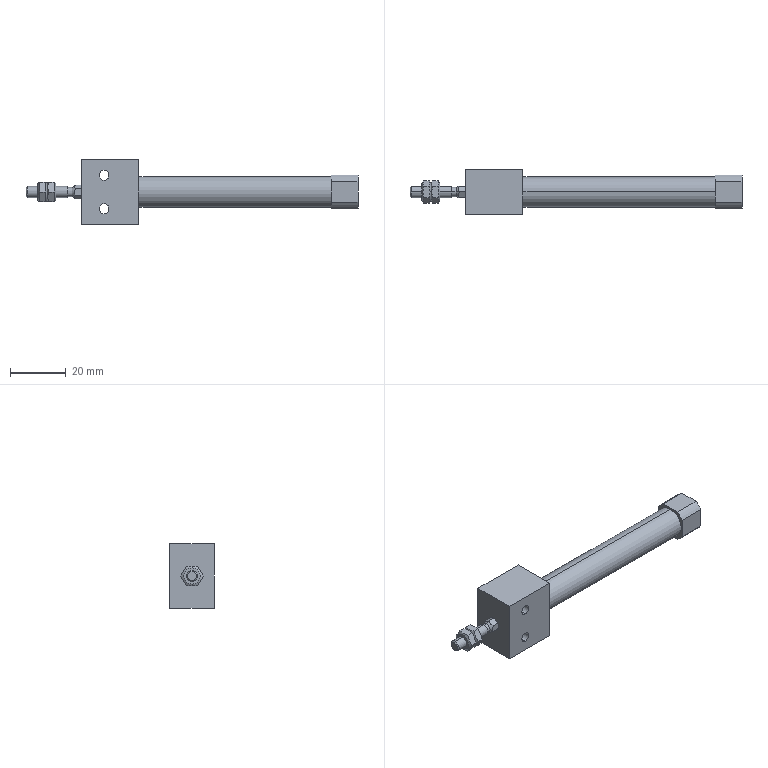Part | STEP file | Mirror CJ2RKA10-45(0_0_0) | 2 solids | 98 faces | box 119 x 16 x 23 mm | volume 12263 mm3 | plane 36 | cylinder 32 | cone 28 | spline 2 | commonest cylinder face diameters 3.242 x4 3.5 x4 4.134 x4 6.5 x4 10 x4 14 x4